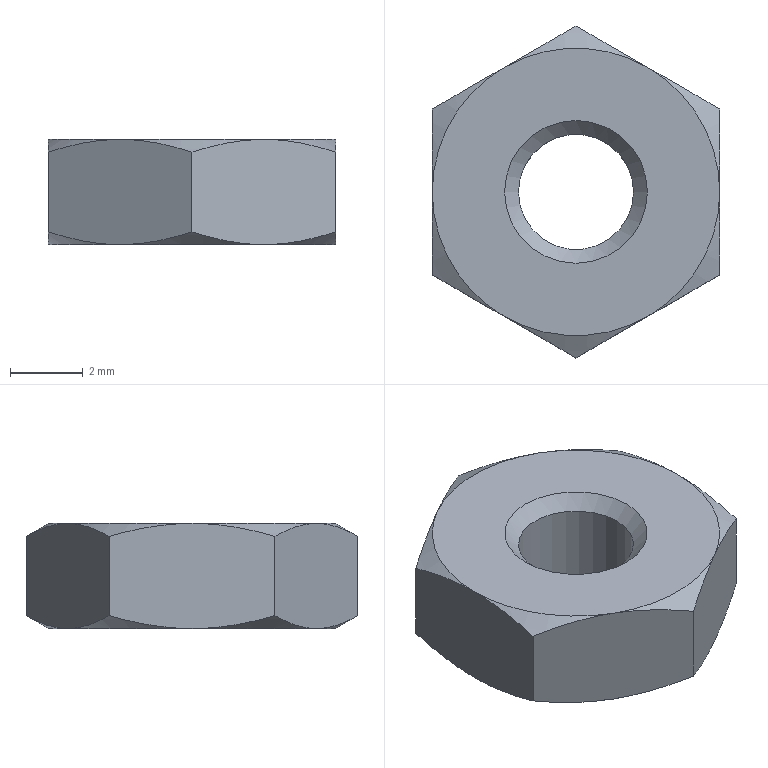Part | NX | features DATUM_CSYS 4, EXTRACT_DATUM_AXIS 4, SKETCH 3, EXTRACT_DATUM_PLANE 2, EXTRACT_FACE 2, EXTRACT_STRING 2, SWP104 2, CHAMFER 1, EXTRUDE 1, Instance Feature 1, Mirror Feature 1 | 1 solid | 23 faces | box 7.925 x 9.151 x 2.896 mm | volume 131.895 mm3 | cone 14 | plane 8 | cylinder 1 | commonest cylinder face diameters 3.175 x1
STEP:
#1=CARTESIAN_POINT('',(1.968,0.,0.));
#2=VERTEX_POINT('',#1);
#3=CARTESIAN_POINT('',(0.,0.,0.));
#4=DIRECTION('',(0.,0.,1.));
#5=DIRECTION('',(1.,0.,0.));
#6=AXIS2_PLACEMENT_3D('',#3,#4,#5);
#7=CIRCLE('',#6,1.968);
#8=EDGE_CURVE('',#2,#2,#7,.T.);
#9=ORIENTED_EDGE('',*,*,#8,.T.);
#10=EDGE_LOOP('',(#9));
#11=FACE_BOUND('',#10,.T.);
#12=CARTESIAN_POINT('',(3.962,0.,0.));
#13=VERTEX_POINT('',#12);
#14=CARTESIAN_POINT('',(1.981,3.432,0.));
#15=VERTEX_POINT('',#14);
#16=CARTESIAN_POINT('',(0.,0.,0.));
#17=DIRECTION('',(0.,0.,1.));
#18=DIRECTION('',(1.,0.,0.));
#19=AXIS2_PLACEMENT_3D('',#16,#17,#18);
#20=CIRCLE('',#19,3.962);
#21=EDGE_CURVE('',#13,#15,#20,.T.);
#22=ORIENTED_EDGE('',*,*,#21,.F.);
#23=CARTESIAN_POINT('',(1.981,-3.432,0.));
#24=VERTEX_POINT('',#23);
#25=CARTESIAN_POINT('',(0.,0.,0.));
#26=DIRECTION('',(0.,0.,1.));
#27=DIRECTION('',(1.,0.,0.));
#28=AXIS2_PLACEMENT_3D('',#25,#26,#27);
#29=CIRCLE('',#28,3.962);
#30=EDGE_CURVE('',#24,#13,#29,.T.);
#31=ORIENTED_EDGE('',*,*,#30,.F.);
#32=CARTESIAN_POINT('',(-1.981,-3.432,0.));
#33=VERTEX_POINT('',#32);
#34=CARTESIAN_POINT('',(0.,0.,0.));
#35=DIRECTION('',(0.,0.,1.));
#36=DIRECTION('',(1.,0.,0.));
#37=AXIS2_PLACEMENT_3D('',#34,#35,#36);
#38=CIRCLE('',#37,3.962);
#39=EDGE_CURVE('',#33,#24,#38,.T.);
#40=ORIENTED_EDGE('',*,*,#39,.F.);
#41=CARTESIAN_POINT('',(-3.962,0.,0.));
#42=VERTEX_POINT('',#41);
#43=CARTESIAN_POINT('',(0.,0.,0.));
#44=DIRECTION('',(0.,0.,1.));
#45=DIRECTION('',(1.,0.,0.));
#46=AXIS2_PLACEMENT_3D('',#43,#44,#45);
#47=CIRCLE('',#46,3.962);
#48=EDGE_CURVE('',#42,#33,#47,.T.);
#49=ORIENTED_EDGE('',*,*,#48,.F.);
#50=CARTESIAN_POINT('',(-1.981,3.432,0.));
#51=VERTEX_POINT('',#50);
#52=CARTESIAN_POINT('',(0.,0.,0.));
#53=DIRECTION('',(0.,0.,1.));
#54=DIRECTION('',(1.,0.,0.));
#55=AXIS2_PLACEMENT_3D('',#52,#53,#54);
#56=CIRCLE('',#55,3.962);
#57=EDGE_CURVE('',#51,#42,#56,.T.);
#58=ORIENTED_EDGE('',*,*,#57,.F.);
#59=CARTESIAN_POINT('',(0.,0.,0.));
#60=DIRECTION('',(0.,0.,1.));
#61=DIRECTION('',(1.,0.,0.));
#62=AXIS2_PLACEMENT_3D('',#59,#60,#61);
#63=CIRCLE('',#62,3.962);
#64=EDGE_CURVE('',#15,#51,#63,.T.);
#65=ORIENTED_EDGE('',*,*,#64,.F.);
#66=EDGE_LOOP('',(#22,#31,#40,#49,#58,#65));
#67=FACE_BOUND('',#66,.T.);
#68=CARTESIAN_POINT('',(0.,0.,0.));
#69=DIRECTION('',(0.,0.,1.));
#70=DIRECTION('',(1.,0.,0.));
#71=AXIS2_PLACEMENT_3D('',#68,#69,#70);
#72=PLANE('',#71);
#73=ADVANCED_FACE('',(#11,#67),#72,.F.);
#74=CARTESIAN_POINT('',(1.968,0.,2.896));
#75=VERTEX_POINT('',#74);
#76=CARTESIAN_POINT('',(0.,0.,2.896));
#77=DIRECTION('',(0.,0.,1.));
#78=DIRECTION('',(1.,0.,0.));
#79=AXIS2_PLACEMENT_3D('',#76,#77,#78);
#80=CIRCLE('',#79,1.968);
#81=EDGE_CURVE('',#75,#75,#80,.F.);
#82=ORIENTED_EDGE('',*,*,#81,.T.);
#83=EDGE_LOOP('',(#82));
#84=FACE_BOUND('',#83,.T.);
#85=CARTESIAN_POINT('',(-3.962,0.,2.896));
#86=VERTEX_POINT('',#85);
#87=CARTESIAN_POINT('',(-1.981,3.432,2.896));
#88=VERTEX_POINT('',#87);
#89=CARTESIAN_POINT('',(0.,0.,2.896));
#90=DIRECTION('',(0.,0.,-1.));
#91=DIRECTION('',(-1.,0.,0.));
#92=AXIS2_PLACEMENT_3D('',#89,#90,#91);
#93=CIRCLE('',#92,3.962);
#94=EDGE_CURVE('',#86,#88,#93,.T.);
#95=ORIENTED_EDGE('',*,*,#94,.F.);
#96=CARTESIAN_POINT('',(-1.981,-3.432,2.896));
#97=VERTEX_POINT('',#96);
#98=CARTESIAN_POINT('',(0.,0.,2.896));
#99=DIRECTION('',(0.,0.,-1.));
#100=DIRECTION('',(-1.,0.,0.));
#101=AXIS2_PLACEMENT_3D('',#98,#99,#100);
#102=CIRCLE('',#101,3.962);
#103=EDGE_CURVE('',#97,#86,#102,.T.);
#104=ORIENTED_EDGE('',*,*,#103,.F.);
#105=CARTESIAN_POINT('',(1.981,-3.432,2.896));
#106=VERTEX_POINT('',#105);
#107=CARTESIAN_POINT('',(0.,0.,2.896));
#108=DIRECTION('',(0.,0.,-1.));
#109=DIRECTION('',(-1.,0.,0.));
#110=AXIS2_PLACEMENT_3D('',#107,#108,#109);
#111=CIRCLE('',#110,3.962);
#112=EDGE_CURVE('',#106,#97,#111,.T.);
#113=ORIENTED_EDGE('',*,*,#112,.F.);
#114=CARTESIAN_POINT('',(3.962,0.,2.896));
#115=VERTEX_POINT('',#114);
#116=CARTESIAN_POINT('',(0.,0.,2.896));
#117=DIRECTION('',(0.,0.,-1.));
#118=DIRECTION('',(-1.,0.,0.));
#119=AXIS2_PLACEMENT_3D('',#116,#117,#118);
#120=CIRCLE('',#119,3.962);
#121=EDGE_CURVE('',#115,#106,#120,.T.);
#122=ORIENTED_EDGE('',*,*,#121,.F.);
#123=CARTESIAN_POINT('',(1.981,3.432,2.896));
#124=VERTEX_POINT('',#123);
#125=CARTESIAN_POINT('',(0.,0.,2.896));
#126=DIRECTION('',(0.,0.,-1.));
#127=DIRECTION('',(-1.,0.,0.));
#128=AXIS2_PLACEMENT_3D('',#125,#126,#127);
#129=CIRCLE('',#128,3.962);
#130=EDGE_CURVE('',#124,#115,#129,.T.);
#131=ORIENTED_EDGE('',*,*,#130,.F.);
#132=CARTESIAN_POINT('',(0.,0.,2.896));
#133=DIRECTION('',(0.,0.,-1.));
#134=DIRECTION('',(-1.,0.,0.));
#135=AXIS2_PLACEMENT_3D('',#132,#133,#134);
#136=CIRCLE('',#135,3.962);
#137=EDGE_CURVE('',#88,#124,#136,.T.);
#138=ORIENTED_EDGE('',*,*,#137,.F.);
#139=EDGE_LOOP('',(#95,#104,#113,#122,#131,#138));
#140=FACE_BOUND('',#139,.T.);
#141=CARTESIAN_POINT('',(0.,0.,2.896));
#142=DIRECTION('',(0.,0.,1.));
#143=DIRECTION('',(1.,0.,0.));
#144=AXIS2_PLACEMENT_3D('',#141,#142,#143);
#145=PLANE('',#144);
#146=ADVANCED_FACE('',(#84,#140),#145,.T.);
#147=CARTESIAN_POINT('',(-3.962,2.288,2.542));
#148=VERTEX_POINT('',#147);
#149=CARTESIAN_POINT('',(-3.962,2.288,0.3539));
#150=VERTEX_POINT('',#149);
#151=CARTESIAN_POINT('',(-3.962,2.288,2.896));
#152=DIRECTION('',(0.,0.,-1.));
#153=VECTOR('',#152,1000.);
#154=LINE('',#151,#153);
#155=EDGE_CURVE('',#148,#150,#154,.T.);
#156=ORIENTED_EDGE('',*,*,#155,.T.);
#157=CARTESIAN_POINT('',(-3.962,0.,0.));
#158=CARTESIAN_POINT('',(-3.962,0.7737,0.));
#159=CARTESIAN_POINT('',(-3.962,1.548,0.1403));
#160=CARTESIAN_POINT('',(-3.962,2.288,0.3539));
#161=B_SPLINE_CURVE_WITH_KNOTS('',3,(#157,#158,#159,#160),.UNSPECIFIED.,.F.,.F.,(4,4),(0.006401,0.008716),.UNSPECIFIED.);
#162=EDGE_CURVE('',#150,#42,#161,.F.);
#163=ORIENTED_EDGE('',*,*,#162,.T.);
#164=CARTESIAN_POINT('',(-3.962,-2.288,0.3539));
#165=VERTEX_POINT('',#164);
#166=CARTESIAN_POINT('',(-3.962,-2.288,0.3539));
#167=CARTESIAN_POINT('',(-3.962,-1.544,0.1391));
#168=CARTESIAN_POINT('',(-3.962,-0.7732,0.));
#169=CARTESIAN_POINT('',(-3.962,0.,0.));
#170=B_SPLINE_CURVE_WITH_KNOTS('',3,(#166,#167,#168,#169),.UNSPECIFIED.,.F.,.F.,(4,4),(0.004086,0.006401),.UNSPECIFIED.);
#171=EDGE_CURVE('',#42,#165,#170,.F.);
#172=ORIENTED_EDGE('',*,*,#171,.T.);
#173=CARTESIAN_POINT('',(-3.962,-2.288,2.542));
#174=VERTEX_POINT('',#173);
#175=CARTESIAN_POINT('',(-3.962,-2.288,2.896));
#176=DIRECTION('',(0.,0.,-1.));
#177=VECTOR('',#176,1000.);
#178=LINE('',#175,#177);
#179=EDGE_CURVE('',#174,#165,#178,.T.);
#180=ORIENTED_EDGE('',*,*,#179,.F.);
#181=CARTESIAN_POINT('',(-3.962,-2.288,2.542));
#182=CARTESIAN_POINT('',(-3.962,-1.544,2.757));
#183=CARTESIAN_POINT('',(-3.962,-0.7732,2.896));
#184=CARTESIAN_POINT('',(-3.962,0.,2.896));
#185=B_SPLINE_CURVE_WITH_KNOTS('',3,(#181,#182,#183,#184),.UNSPECIFIED.,.F.,.F.,(4,4),(0.004086,0.006401),.UNSPECIFIED.);
#186=EDGE_CURVE('',#174,#86,#185,.T.);
#187=ORIENTED_EDGE('',*,*,#186,.T.);
#188=CARTESIAN_POINT('',(-3.962,0.,2.896));
#189=CARTESIAN_POINT('',(-3.962,0.7737,2.896));
#190=CARTESIAN_POINT('',(-3.962,1.548,2.755));
#191=CARTESIAN_POINT('',(-3.962,2.288,2.542));
#192=B_SPLINE_CURVE_WITH_KNOTS('',3,(#188,#189,#190,#191),.UNSPECIFIED.,.F.,.F.,(4,4),(0.006401,0.008716),.UNSPECIFIED.);
#193=EDGE_CURVE('',#86,#148,#192,.T.);
#194=ORIENTED_EDGE('',*,*,#193,.T.);
#195=EDGE_LOOP('',(#156,#163,#172,#180,#187,#194));
#196=FACE_BOUND('',#195,.T.);
#197=CARTESIAN_POINT('',(-3.962,2.288,2.896));
#198=DIRECTION('',(1.,0.,0.));
#199=DIRECTION('',(0.,1.,0.));
#200=AXIS2_PLACEMENT_3D('',#197,#198,#199);
#201=PLANE('',#200);
#202=ADVANCED_FACE('',(#196),#201,.F.);
#203=ORIENTED_EDGE('',*,*,#179,.T.);
#204=CARTESIAN_POINT('',(-3.962,-2.288,0.3539));
#205=CARTESIAN_POINT('',(-3.314,-2.662,0.1378));
#206=CARTESIAN_POINT('',(-2.656,-3.042,0.));
#207=CARTESIAN_POINT('',(-1.981,-3.432,0.));
#208=B_SPLINE_CURVE_WITH_KNOTS('',3,(#204,#205,#206,#207),.UNSPECIFIED.,.F.,.F.,(4,4),(0.000000238,0.002315),.UNSPECIFIED.);
#209=EDGE_CURVE('',#165,#33,#208,.T.);
#210=ORIENTED_EDGE('',*,*,#209,.T.);
#211=CARTESIAN_POINT('',(0.,-4.575,0.3539));
#212=VERTEX_POINT('',#211);
#213=CARTESIAN_POINT('',(-1.981,-3.432,0.));
#214=CARTESIAN_POINT('',(-1.309,-3.82,0.));
#215=CARTESIAN_POINT('',(-0.6466,-4.202,0.1384));
#216=CARTESIAN_POINT('',(0.,-4.575,0.3539));
#217=B_SPLINE_CURVE_WITH_KNOTS('',3,(#213,#214,#215,#216),.UNSPECIFIED.,.F.,.F.,(4,4),(0.002315,0.004621),.UNSPECIFIED.);
#218=EDGE_CURVE('',#33,#212,#217,.T.);
#219=ORIENTED_EDGE('',*,*,#218,.T.);
#220=CARTESIAN_POINT('',(0.,-4.575,2.542));
#221=VERTEX_POINT('',#220);
#222=CARTESIAN_POINT('',(0.,-4.575,2.896));
#223=DIRECTION('',(0.,0.,-1.));
#224=VECTOR('',#223,1000.);
#225=LINE('',#222,#224);
#226=EDGE_CURVE('',#221,#212,#225,.T.);
#227=ORIENTED_EDGE('',*,*,#226,.F.);
#228=CARTESIAN_POINT('',(0.,-4.575,2.542));
#229=CARTESIAN_POINT('',(-0.6482,-4.201,2.758));
#230=CARTESIAN_POINT('',(-1.306,-3.821,2.896));
#231=CARTESIAN_POINT('',(-1.981,-3.432,2.896));
#232=B_SPLINE_CURVE_WITH_KNOTS('',3,(#228,#229,#230,#231),.UNSPECIFIED.,.F.,.F.,(4,4),(0.000000238,0.002315),.UNSPECIFIED.);
#233=EDGE_CURVE('',#221,#97,#232,.T.);
#234=ORIENTED_EDGE('',*,*,#233,.T.);
#235=CARTESIAN_POINT('',(-1.981,-3.432,2.896));
#236=CARTESIAN_POINT('',(-2.654,-3.043,2.896));
#237=CARTESIAN_POINT('',(-3.316,-2.661,2.757));
#238=CARTESIAN_POINT('',(-3.962,-2.288,2.542));
#239=B_SPLINE_CURVE_WITH_KNOTS('',3,(#235,#236,#237,#238),.UNSPECIFIED.,.F.,.F.,(4,4),(0.002315,0.004621),.UNSPECIFIED.);
#240=EDGE_CURVE('',#97,#174,#239,.T.);
#241=ORIENTED_EDGE('',*,*,#240,.T.);
#242=EDGE_LOOP('',(#203,#210,#219,#227,#234,#241));
#243=FACE_BOUND('',#242,.T.);
#244=CARTESIAN_POINT('',(-3.962,-2.288,2.896));
#245=DIRECTION('',(0.5,0.866,0.));
#246=DIRECTION('',(-0.866,0.5,0.));
#247=AXIS2_PLACEMENT_3D('',#244,#245,#246);
#248=PLANE('',#247);
#249=ADVANCED_FACE('',(#243),#248,.F.);
#250=ORIENTED_EDGE('',*,*,#226,.T.);
#251=CARTESIAN_POINT('',(0.,-4.575,0.3539));
#252=CARTESIAN_POINT('',(0.6482,-4.201,0.1378));
#253=CARTESIAN_POINT('',(1.306,-3.821,0.));
#254=CARTESIAN_POINT('',(1.981,-3.432,0.));
#255=B_SPLINE_CURVE_WITH_KNOTS('',3,(#251,#252,#253,#254),.UNSPECIFIED.,.F.,.F.,(4,4),(0.000000238,0.002315),.UNSPECIFIED.);
#256=EDGE_CURVE('',#212,#24,#255,.T.);
#257=ORIENTED_EDGE('',*,*,#256,.T.);
#258=CARTESIAN_POINT('',(3.962,-2.288,0.3539));
#259=VERTEX_POINT('',#258);
#260=CARTESIAN_POINT('',(1.981,-3.432,0.));
#261=CARTESIAN_POINT('',(2.654,-3.043,0.));
#262=CARTESIAN_POINT('',(3.316,-2.661,0.1384));
#263=CARTESIAN_POINT('',(3.962,-2.288,0.3539));
#264=B_SPLINE_CURVE_WITH_KNOTS('',3,(#260,#261,#262,#263),.UNSPECIFIED.,.F.,.F.,(4,4),(0.002315,0.004621),.UNSPECIFIED.);
#265=EDGE_CURVE('',#24,#259,#264,.T.);
#266=ORIENTED_EDGE('',*,*,#265,.T.);
#267=CARTESIAN_POINT('',(3.962,-2.288,2.542));
#268=VERTEX_POINT('',#267);
#269=CARTESIAN_POINT('',(3.962,-2.288,2.896));
#270=DIRECTION('',(0.,0.,-1.));
#271=VECTOR('',#270,1000.);
#272=LINE('',#269,#271);
#273=EDGE_CURVE('',#268,#259,#272,.T.);
#274=ORIENTED_EDGE('',*,*,#273,.F.);
#275=CARTESIAN_POINT('',(3.962,-2.288,2.542));
#276=CARTESIAN_POINT('',(3.314,-2.662,2.758));
#277=CARTESIAN_POINT('',(2.656,-3.042,2.896));
#278=CARTESIAN_POINT('',(1.981,-3.432,2.896));
#279=B_SPLINE_CURVE_WITH_KNOTS('',3,(#275,#276,#277,#278),.UNSPECIFIED.,.F.,.F.,(4,4),(0.000000238,0.002315),.UNSPECIFIED.);
#280=EDGE_CURVE('',#268,#106,#279,.T.);
#281=ORIENTED_EDGE('',*,*,#280,.T.);
#282=CARTESIAN_POINT('',(1.981,-3.432,2.896));
#283=CARTESIAN_POINT('',(1.309,-3.82,2.896));
#284=CARTESIAN_POINT('',(0.6466,-4.202,2.757));
#285=CARTESIAN_POINT('',(0.,-4.575,2.542));
#286=B_SPLINE_CURVE_WITH_KNOTS('',3,(#282,#283,#284,#285),.UNSPECIFIED.,.F.,.F.,(4,4),(0.002315,0.004621),.UNSPECIFIED.);
#287=EDGE_CURVE('',#106,#221,#286,.T.);
#288=ORIENTED_EDGE('',*,*,#287,.T.);
#289=EDGE_LOOP('',(#250,#257,#266,#274,#281,#288));
#290=FACE_BOUND('',#289,.T.);
#291=CARTESIAN_POINT('',(0.,-4.575,2.896));
#292=DIRECTION('',(-0.5,0.866,0.));
#293=DIRECTION('',(-0.866,-0.5,0.));
#294=AXIS2_PLACEMENT_3D('',#291,#292,#293);
#295=PLANE('',#294);
#296=ADVANCED_FACE('',(#290),#295,.F.);
#297=ORIENTED_EDGE('',*,*,#273,.T.);
#298=CARTESIAN_POINT('',(3.962,-2.288,0.3539));
#299=CARTESIAN_POINT('',(3.962,-1.544,0.1391));
#300=CARTESIAN_POINT('',(3.962,-0.7732,0.));
#301=CARTESIAN_POINT('',(3.962,0.,0.));
#302=B_SPLINE_CURVE_WITH_KNOTS('',3,(#298,#299,#300,#301),.UNSPECIFIED.,.F.,.F.,(4,4),(0.004086,0.006401),.UNSPECIFIED.);
#303=EDGE_CURVE('',#259,#13,#302,.T.);
#304=ORIENTED_EDGE('',*,*,#303,.T.);
#305=CARTESIAN_POINT('',(3.962,2.288,0.3539));
#306=VERTEX_POINT('',#305);
#307=CARTESIAN_POINT('',(3.962,0.,0.));
#308=CARTESIAN_POINT('',(3.962,0.7737,0.));
#309=CARTESIAN_POINT('',(3.962,1.548,0.1403));
#310=CARTESIAN_POINT('',(3.962,2.288,0.3539));
#311=B_SPLINE_CURVE_WITH_KNOTS('',3,(#307,#308,#309,#310),.UNSPECIFIED.,.F.,.F.,(4,4),(0.006401,0.008716),.UNSPECIFIED.);
#312=EDGE_CURVE('',#13,#306,#311,.T.);
#313=ORIENTED_EDGE('',*,*,#312,.T.);
#314=CARTESIAN_POINT('',(3.962,2.288,2.542));
#315=VERTEX_POINT('',#314);
#316=CARTESIAN_POINT('',(3.962,2.288,2.896));
#317=DIRECTION('',(0.,0.,-1.));
#318=VECTOR('',#317,1000.);
#319=LINE('',#316,#318);
#320=EDGE_CURVE('',#315,#306,#319,.T.);
#321=ORIENTED_EDGE('',*,*,#320,.F.);
#322=CARTESIAN_POINT('',(3.962,0.,2.896));
#323=CARTESIAN_POINT('',(3.962,0.7737,2.896));
#324=CARTESIAN_POINT('',(3.962,1.548,2.755));
#325=CARTESIAN_POINT('',(3.962,2.288,2.542));
#326=B_SPLINE_CURVE_WITH_KNOTS('',3,(#322,#323,#324,#325),.UNSPECIFIED.,.F.,.F.,(4,4),(0.006401,0.008716),.UNSPECIFIED.);
#327=EDGE_CURVE('',#315,#115,#326,.F.);
#328=ORIENTED_EDGE('',*,*,#327,.T.);
#329=CARTESIAN_POINT('',(3.962,-2.288,2.542));
#330=CARTESIAN_POINT('',(3.962,-1.544,2.757));
#331=CARTESIAN_POINT('',(3.962,-0.7732,2.896));
#332=CARTESIAN_POINT('',(3.962,0.,2.896));
#333=B_SPLINE_CURVE_WITH_KNOTS('',3,(#329,#330,#331,#332),.UNSPECIFIED.,.F.,.F.,(4,4),(0.004086,0.006401),.UNSPECIFIED.);
#334=EDGE_CURVE('',#115,#268,#333,.F.);
#335=ORIENTED_EDGE('',*,*,#334,.T.);
#336=EDGE_LOOP('',(#297,#304,#313,#321,#328,#335));
#337=FACE_BOUND('',#336,.T.);
#338=CARTESIAN_POINT('',(3.962,-2.288,2.896));
#339=DIRECTION('',(-1.,0.,0.));
#340=DIRECTION('',(0.,-1.,0.));
#341=AXIS2_PLACEMENT_3D('',#338,#339,#340);
#342=PLANE('',#341);
#343=ADVANCED_FACE('',(#337),#342,.F.);
#344=ORIENTED_EDGE('',*,*,#320,.T.);
#345=CARTESIAN_POINT('',(3.962,2.288,0.3539));
#346=CARTESIAN_POINT('',(3.314,2.662,0.1378));
#347=CARTESIAN_POINT('',(2.656,3.042,0.));
#348=CARTESIAN_POINT('',(1.981,3.432,0.));
#349=B_SPLINE_CURVE_WITH_KNOTS('',3,(#345,#346,#347,#348),.UNSPECIFIED.,.F.,.F.,(4,4),(0.000000238,0.002315),.UNSPECIFIED.);
#350=EDGE_CURVE('',#306,#15,#349,.T.);
#351=ORIENTED_EDGE('',*,*,#350,.T.);
#352=CARTESIAN_POINT('',(0.,4.575,0.3539));
#353=VERTEX_POINT('',#352);
#354=CARTESIAN_POINT('',(1.981,3.432,0.));
#355=CARTESIAN_POINT('',(1.309,3.82,0.));
#356=CARTESIAN_POINT('',(0.6466,4.202,0.1384));
#357=CARTESIAN_POINT('',(0.,4.575,0.3539));
#358=B_SPLINE_CURVE_WITH_KNOTS('',3,(#354,#355,#356,#357),.UNSPECIFIED.,.F.,.F.,(4,4),(0.002315,0.004621),.UNSPECIFIED.);
#359=EDGE_CURVE('',#15,#353,#358,.T.);
#360=ORIENTED_EDGE('',*,*,#359,.T.);
#361=CARTESIAN_POINT('',(0.,4.575,2.542));
#362=VERTEX_POINT('',#361);
#363=CARTESIAN_POINT('',(0.,4.575,2.896));
#364=DIRECTION('',(0.,0.,-1.));
#365=VECTOR('',#364,1000.);
#366=LINE('',#363,#365);
#367=EDGE_CURVE('',#362,#353,#366,.T.);
#368=ORIENTED_EDGE('',*,*,#367,.F.);
#369=CARTESIAN_POINT('',(0.,4.575,2.542));
#370=CARTESIAN_POINT('',(0.6482,4.201,2.758));
#371=CARTESIAN_POINT('',(1.306,3.821,2.896));
#372=CARTESIAN_POINT('',(1.981,3.432,2.896));
#373=B_SPLINE_CURVE_WITH_KNOTS('',3,(#369,#370,#371,#372),.UNSPECIFIED.,.F.,.F.,(4,4),(0.000000238,0.002315),.UNSPECIFIED.);
#374=EDGE_CURVE('',#362,#124,#373,.T.);
#375=ORIENTED_EDGE('',*,*,#374,.T.);
#376=CARTESIAN_POINT('',(1.981,3.432,2.896));
#377=CARTESIAN_POINT('',(2.654,3.043,2.896));
#378=CARTESIAN_POINT('',(3.316,2.661,2.757));
#379=CARTESIAN_POINT('',(3.962,2.288,2.542));
#380=B_SPLINE_CURVE_WITH_KNOTS('',3,(#376,#377,#378,#379),.UNSPECIFIED.,.F.,.F.,(4,4),(0.002315,0.004621),.UNSPECIFIED.);
#381=EDGE_CURVE('',#124,#315,#380,.T.);
#382=ORIENTED_EDGE('',*,*,#381,.T.);
#383=EDGE_LOOP('',(#344,#351,#360,#368,#375,#382));
#384=FACE_BOUND('',#383,.T.);
#385=CARTESIAN_POINT('',(3.962,2.288,2.896));
#386=DIRECTION('',(-0.5,-0.866,0.));
#387=DIRECTION('',(0.866,-0.5,0.));
#388=AXIS2_PLACEMENT_3D('',#385,#386,#387);
#389=PLANE('',#388);
#390=ADVANCED_FACE('',(#384),#389,.F.);
#391=ORIENTED_EDGE('',*,*,#367,.T.);
#392=CARTESIAN_POINT('',(0.,4.575,0.3539));
#393=CARTESIAN_POINT('',(-0.6482,4.201,0.1378));
#394=CARTESIAN_POINT('',(-1.306,3.821,0.));
#395=CARTESIAN_POINT('',(-1.981,3.432,0.));
#396=B_SPLINE_CURVE_WITH_KNOTS('',3,(#392,#393,#394,#395),.UNSPECIFIED.,.F.,.F.,(4,4),(0.000000238,0.002315),.UNSPECIFIED.);
#397=EDGE_CURVE('',#353,#51,#396,.T.);
#398=ORIENTED_EDGE('',*,*,#397,.T.);
#399=CARTESIAN_POINT('',(-1.981,3.432,0.));
#400=CARTESIAN_POINT('',(-2.654,3.043,0.));
#401=CARTESIAN_POINT('',(-3.316,2.661,0.1384));
#402=CARTESIAN_POINT('',(-3.962,2.288,0.3539));
#403=B_SPLINE_CURVE_WITH_KNOTS('',3,(#399,#400,#401,#402),.UNSPECIFIED.,.F.,.F.,(4,4),(0.002315,0.004621),.UNSPECIFIED.);
#404=EDGE_CURVE('',#51,#150,#403,.T.);
#405=ORIENTED_EDGE('',*,*,#404,.T.);
#406=ORIENTED_EDGE('',*,*,#155,.F.);
#407=CARTESIAN_POINT('',(-3.962,2.288,2.542));
#408=CARTESIAN_POINT('',(-3.314,2.662,2.758));
#409=CARTESIAN_POINT('',(-2.656,3.042,2.896));
#410=CARTESIAN_POINT('',(-1.981,3.432,2.896));
#411=B_SPLINE_CURVE_WITH_KNOTS('',3,(#407,#408,#409,#410),.UNSPECIFIED.,.F.,.F.,(4,4),(0.000000238,0.002315),.UNSPECIFIED.);
#412=EDGE_CURVE('',#148,#88,#411,.T.);
#413=ORIENTED_EDGE('',*,*,#412,.T.);
#414=CARTESIAN_POINT('',(-1.981,3.432,2.896));
#415=CARTESIAN_POINT('',(-1.309,3.82,2.896));
#416=CARTESIAN_POINT('',(-0.6466,4.202,2.757));
#417=CARTESIAN_POINT('',(0.,4.575,2.542));
#418=B_SPLINE_CURVE_WITH_KNOTS('',3,(#414,#415,#416,#417),.UNSPECIFIED.,.F.,.F.,(4,4),(0.002315,0.004621),.UNSPECIFIED.);
#419=EDGE_CURVE('',#88,#362,#418,.T.);
#420=ORIENTED_EDGE('',*,*,#419,.T.);
#421=EDGE_LOOP('',(#391,#398,#405,#406,#413,#420));
#422=FACE_BOUND('',#421,.T.);
#423=CARTESIAN_POINT('',(0.,4.575,2.896));
#424=DIRECTION('',(0.5,-0.866,0.));
#425=DIRECTION('',(0.866,0.5,0.));
#426=AXIS2_PLACEMENT_3D('',#423,#424,#425);
#427=PLANE('',#426);
#428=ADVANCED_FACE('',(#422),#427,.F.);
#429=CARTESIAN_POINT('',(1.587,0.,0.381));
#430=VERTEX_POINT('',#429);
#431=CARTESIAN_POINT('',(0.,0.,0.381));
#432=DIRECTION('',(0.,0.,1.));
#433=DIRECTION('',(1.,0.,0.));
#434=AXIS2_PLACEMENT_3D('',#431,#432,#433);
#435=CIRCLE('',#434,1.587);
#436=EDGE_CURVE('',#430,#430,#435,.F.);
#437=ORIENTED_EDGE('',*,*,#436,.T.);
#438=EDGE_LOOP('',(#437));
#439=FACE_BOUND('',#438,.T.);
#440=CARTESIAN_POINT('',(1.587,0.,2.515));
#441=VERTEX_POINT('',#440);
#442=CARTESIAN_POINT('',(0.,0.,2.515));
#443=DIRECTION('',(0.,0.,1.));
#444=DIRECTION('',(1.,0.,0.));
#445=AXIS2_PLACEMENT_3D('',#442,#443,#444);
#446=CIRCLE('',#445,1.587);
#447=EDGE_CURVE('',#441,#441,#446,.T.);
#448=ORIENTED_EDGE('',*,*,#447,.T.);
#449=EDGE_LOOP('',(#448));
#450=FACE_BOUND('',#449,.T.);
#451=CARTESIAN_POINT('',(0.,0.,2.896));
#452=DIRECTION('',(0.,0.,-1.));
#453=DIRECTION('',(-1.,0.,0.));
#454=AXIS2_PLACEMENT_3D('',#451,#452,#453);
#455=CYLINDRICAL_SURFACE('',#454,1.587);
#456=ADVANCED_FACE('',(#439,#450),#455,.F.);
#457=ORIENTED_EDGE('',*,*,#419,.F.);
#458=ORIENTED_EDGE('',*,*,#137,.T.);
#459=ORIENTED_EDGE('',*,*,#374,.F.);
#460=EDGE_LOOP('',(#457,#458,#459));
#461=FACE_BOUND('',#460,.T.);
#462=CARTESIAN_POINT('',(0.,0.,2.896));
#463=DIRECTION('',(0.,0.,-1.));
#464=DIRECTION('',(-1.,0.,0.));
#465=AXIS2_PLACEMENT_3D('',#462,#463,#464);
#466=CONICAL_SURFACE('',#465,3.962,1.047);
#467=ADVANCED_FACE('',(#461),#466,.T.);
#468=ORIENTED_EDGE('',*,*,#94,.T.);
#469=ORIENTED_EDGE('',*,*,#412,.F.);
#470=ORIENTED_EDGE('',*,*,#193,.F.);
#471=EDGE_LOOP('',(#468,#469,#470));
#472=FACE_BOUND('',#471,.T.);
#473=CARTESIAN_POINT('',(0.,0.,2.896));
#474=DIRECTION('',(0.,0.,-1.));
#475=DIRECTION('',(-1.,0.,0.));
#476=AXIS2_PLACEMENT_3D('',#473,#474,#475);
#477=CONICAL_SURFACE('',#476,3.962,1.047);
#478=ADVANCED_FACE('',(#472),#477,.T.);
#479=ORIENTED_EDGE('',*,*,#381,.F.);
#480=ORIENTED_EDGE('',*,*,#130,.T.);
#481=ORIENTED_EDGE('',*,*,#327,.F.);
#482=EDGE_LOOP('',(#479,#480,#481));
#483=FACE_BOUND('',#482,.T.);
#484=CARTESIAN_POINT('',(0.,0.,2.896));
#485=DIRECTION('',(0.,0.,-1.));
#486=DIRECTION('',(-1.,0.,0.));
#487=AXIS2_PLACEMENT_3D('',#484,#485,#486);
#488=CONICAL_SURFACE('',#487,3.962,1.047);
#489=ADVANCED_FACE('',(#483),#488,.T.);
#490=ORIENTED_EDGE('',*,*,#334,.F.);
#491=ORIENTED_EDGE('',*,*,#121,.T.);
#492=ORIENTED_EDGE('',*,*,#280,.F.);
#493=EDGE_LOOP('',(#490,#491,#492));
#494=FACE_BOUND('',#493,.T.);
#495=CARTESIAN_POINT('',(0.,0.,2.896));
#496=DIRECTION('',(0.,0.,-1.));
#497=DIRECTION('',(-1.,0.,0.));
#498=AXIS2_PLACEMENT_3D('',#495,#496,#497);
#499=CONICAL_SURFACE('',#498,3.962,1.047);
#500=ADVANCED_FACE('',(#494),#499,.T.);
#501=ORIENTED_EDGE('',*,*,#112,.T.);
#502=ORIENTED_EDGE('',*,*,#233,.F.);
#503=ORIENTED_EDGE('',*,*,#287,.F.);
#504=EDGE_LOOP('',(#501,#502,#503));
#505=FACE_BOUND('',#504,.T.);
#506=CARTESIAN_POINT('',(0.,0.,2.896));
#507=DIRECTION('',(0.,0.,-1.));
#508=DIRECTION('',(-1.,0.,0.));
#509=AXIS2_PLACEMENT_3D('',#506,#507,#508);
#510=CONICAL_SURFACE('',#509,3.962,1.047);
#511=ADVANCED_FACE('',(#505),#510,.T.);
#512=ORIENTED_EDGE('',*,*,#103,.T.);
#513=ORIENTED_EDGE('',*,*,#186,.F.);
#514=ORIENTED_EDGE('',*,*,#240,.F.);
#515=EDGE_LOOP('',(#512,#513,#514));
#516=FACE_BOUND('',#515,.T.);
#517=CARTESIAN_POINT('',(0.,0.,2.896));
#518=DIRECTION('',(0.,0.,-1.));
#519=DIRECTION('',(-1.,0.,0.));
#520=AXIS2_PLACEMENT_3D('',#517,#518,#519);
#521=CONICAL_SURFACE('',#520,3.962,1.047);
#522=ADVANCED_FACE('',(#516),#521,.T.);
#523=ORIENTED_EDGE('',*,*,#404,.F.);
#524=ORIENTED_EDGE('',*,*,#57,.T.);
#525=ORIENTED_EDGE('',*,*,#162,.F.);
#526=EDGE_LOOP('',(#523,#524,#525));
#527=FACE_BOUND('',#526,.T.);
#528=CARTESIAN_POINT('',(0.,0.,0.));
#529=DIRECTION('',(0.,0.,1.));
#530=DIRECTION('',(1.,0.,0.));
#531=AXIS2_PLACEMENT_3D('',#528,#529,#530);
#532=CONICAL_SURFACE('',#531,3.962,1.047);
#533=ADVANCED_FACE('',(#527),#532,.T.);
#534=ORIENTED_EDGE('',*,*,#64,.T.);
#535=ORIENTED_EDGE('',*,*,#397,.F.);
#536=ORIENTED_EDGE('',*,*,#359,.F.);
#537=EDGE_LOOP('',(#534,#535,#536));
#538=FACE_BOUND('',#537,.T.);
#539=CARTESIAN_POINT('',(0.,0.,0.));
#540=DIRECTION('',(0.,0.,1.));
#541=DIRECTION('',(1.,0.,0.));
#542=AXIS2_PLACEMENT_3D('',#539,#540,#541);
#543=CONICAL_SURFACE('',#542,3.962,1.047);
#544=ADVANCED_FACE('',(#538),#543,.T.);
#545=ORIENTED_EDGE('',*,*,#21,.T.);
#546=ORIENTED_EDGE('',*,*,#350,.F.);
#547=ORIENTED_EDGE('',*,*,#312,.F.);
#548=EDGE_LOOP('',(#545,#546,#547));
#549=FACE_BOUND('',#548,.T.);
#550=CARTESIAN_POINT('',(0.,0.,0.));
#551=DIRECTION('',(0.,0.,1.));
#552=DIRECTION('',(1.,0.,0.));
#553=AXIS2_PLACEMENT_3D('',#550,#551,#552);
#554=CONICAL_SURFACE('',#553,3.962,1.047);
#555=ADVANCED_FACE('',(#549),#554,.T.);
#556=ORIENTED_EDGE('',*,*,#30,.T.);
#557=ORIENTED_EDGE('',*,*,#303,.F.);
#558=ORIENTED_EDGE('',*,*,#265,.F.);
#559=EDGE_LOOP('',(#556,#557,#558));
#560=FACE_BOUND('',#559,.T.);
#561=CARTESIAN_POINT('',(0.,0.,0.));
#562=DIRECTION('',(0.,0.,1.));
#563=DIRECTION('',(1.,0.,0.));
#564=AXIS2_PLACEMENT_3D('',#561,#562,#563);
#565=CONICAL_SURFACE('',#564,3.962,1.047);
#566=ADVANCED_FACE('',(#560),#565,.T.);
#567=ORIENTED_EDGE('',*,*,#39,.T.);
#568=ORIENTED_EDGE('',*,*,#256,.F.);
#569=ORIENTED_EDGE('',*,*,#218,.F.);
#570=EDGE_LOOP('',(#567,#568,#569));
#571=FACE_BOUND('',#570,.T.);
#572=CARTESIAN_POINT('',(0.,0.,0.));
#573=DIRECTION('',(0.,0.,1.));
#574=DIRECTION('',(1.,0.,0.));
#575=AXIS2_PLACEMENT_3D('',#572,#573,#574);
#576=CONICAL_SURFACE('',#575,3.962,1.047);
#577=ADVANCED_FACE('',(#571),#576,.T.);
#578=ORIENTED_EDGE('',*,*,#48,.T.);
#579=ORIENTED_EDGE('',*,*,#209,.F.);
#580=ORIENTED_EDGE('',*,*,#171,.F.);
#581=EDGE_LOOP('',(#578,#579,#580));
#582=FACE_BOUND('',#581,.T.);
#583=CARTESIAN_POINT('',(0.,0.,0.));
#584=DIRECTION('',(0.,0.,1.));
#585=DIRECTION('',(1.,0.,0.));
#586=AXIS2_PLACEMENT_3D('',#583,#584,#585);
#587=CONICAL_SURFACE('',#586,3.962,1.047);
#588=ADVANCED_FACE('',(#582),#587,.T.);
#589=ORIENTED_EDGE('',*,*,#436,.F.);
#590=EDGE_LOOP('',(#589));
#591=FACE_BOUND('',#590,.T.);
#592=ORIENTED_EDGE('',*,*,#8,.F.);
#593=EDGE_LOOP('',(#592));
#594=FACE_BOUND('',#593,.T.);
#595=CARTESIAN_POINT('',(0.,0.,0.));
#596=DIRECTION('',(0.,0.,-1.));
#597=DIRECTION('',(-1.,0.,0.));
#598=AXIS2_PLACEMENT_3D('',#595,#596,#597);
#599=CONICAL_SURFACE('',#598,1.968,0.7854);
#600=ADVANCED_FACE('',(#591,#594),#599,.F.);
#601=ORIENTED_EDGE('',*,*,#81,.F.);
#602=EDGE_LOOP('',(#601));
#603=FACE_BOUND('',#602,.T.);
#604=ORIENTED_EDGE('',*,*,#447,.F.);
#605=EDGE_LOOP('',(#604));
#606=FACE_BOUND('',#605,.T.);
#607=CARTESIAN_POINT('',(0.,0.,2.515));
#608=DIRECTION('',(0.,0.,1.));
#609=DIRECTION('',(1.,0.,0.));
#610=AXIS2_PLACEMENT_3D('',#607,#608,#609);
#611=CONICAL_SURFACE('',#610,1.587,0.7854);
#612=ADVANCED_FACE('',(#603,#606),#611,.F.);
#613=CLOSED_SHELL('',(#73,#146,#202,#249,#296,#343,#390,#428,#456,#467,#478,#489,#500,#511,#522,#533,#544,#555,#566,#577,#588,#600,#612));
#614=MANIFOLD_SOLID_BREP('',#613);
#615=(LENGTH_UNIT()NAMED_UNIT(*)SI_UNIT(.MILLI.,.METRE.));
#616=UNCERTAINTY_MEASURE_WITH_UNIT(LENGTH_MEASURE(0.0508),#615,'','');
#617=(NAMED_UNIT(*)PLANE_ANGLE_UNIT()SI_UNIT($,.RADIAN.));
#618=(NAMED_UNIT(*)SI_UNIT($,.STERADIAN.)SOLID_ANGLE_UNIT());
#619=(GEOMETRIC_REPRESENTATION_CONTEXT(3)GLOBAL_UNCERTAINTY_ASSIGNED_CONTEXT((#616))GLOBAL_UNIT_ASSIGNED_CONTEXT((#615,#617,#618))REPRESENTATION_CONTEXT('',''));
#620=ADVANCED_BREP_SHAPE_REPRESENTATION('',(#614),#619);